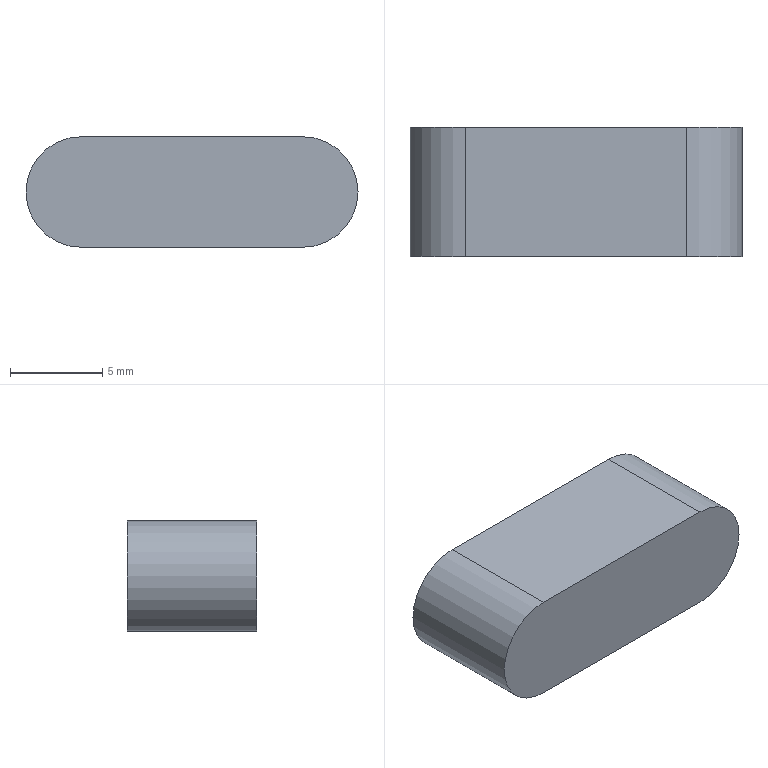Part | NX | features BREP 1 | 1 solid | 6 faces | box 18 x 7 x 6 mm | volume 701.92 mm3 | plane 4 | cylinder 2 | commonest cylinder face diameters 6 x2
STEP:
#1=CARTESIAN_POINT('',(0.,0.,-3.));
#2=VERTEX_POINT('',#1);
#3=CARTESIAN_POINT('',(0.,0.,3.));
#4=VERTEX_POINT('',#3);
#5=CARTESIAN_POINT('',(0.,0.,0.));
#6=DIRECTION('',(0.,1.,0.));
#7=DIRECTION('',(0.,0.,1.));
#8=AXIS2_PLACEMENT_3D('',#5,#6,#7);
#9=CIRCLE('',#8,3.);
#10=EDGE_CURVE('',#2,#4,#9,.T.);
#11=ORIENTED_EDGE('',*,*,#10,.T.);
#12=CARTESIAN_POINT('',(0.,7.,3.));
#13=VERTEX_POINT('',#12);
#14=CARTESIAN_POINT('',(0.,7.,3.));
#15=DIRECTION('',(0.,-1.,0.));
#16=VECTOR('',#15,1000.);
#17=LINE('',#14,#16);
#18=EDGE_CURVE('',#13,#4,#17,.T.);
#19=ORIENTED_EDGE('',*,*,#18,.F.);
#20=CARTESIAN_POINT('',(0.,7.,-3.));
#21=VERTEX_POINT('',#20);
#22=CARTESIAN_POINT('',(0.,7.,0.));
#23=DIRECTION('',(0.,1.,0.));
#24=DIRECTION('',(0.,0.,1.));
#25=AXIS2_PLACEMENT_3D('',#22,#23,#24);
#26=CIRCLE('',#25,3.);
#27=EDGE_CURVE('',#21,#13,#26,.T.);
#28=ORIENTED_EDGE('',*,*,#27,.F.);
#29=CARTESIAN_POINT('',(0.,7.,-3.));
#30=DIRECTION('',(0.,-1.,0.));
#31=VECTOR('',#30,1000.);
#32=LINE('',#29,#31);
#33=EDGE_CURVE('',#21,#2,#32,.T.);
#34=ORIENTED_EDGE('',*,*,#33,.T.);
#35=EDGE_LOOP('',(#11,#19,#28,#34));
#36=FACE_BOUND('',#35,.T.);
#37=CARTESIAN_POINT('',(0.,7.,0.));
#38=DIRECTION('',(0.,-1.,0.));
#39=DIRECTION('',(0.,0.,1.));
#40=AXIS2_PLACEMENT_3D('',#37,#38,#39);
#41=CYLINDRICAL_SURFACE('',#40,3.);
#42=ADVANCED_FACE('',(#36),#41,.T.);
#43=CARTESIAN_POINT('',(12.,0.,3.));
#44=VERTEX_POINT('',#43);
#45=CARTESIAN_POINT('',(0.,0.,3.));
#46=DIRECTION('',(1.,0.,0.));
#47=VECTOR('',#46,1000.);
#48=LINE('',#45,#47);
#49=EDGE_CURVE('',#4,#44,#48,.T.);
#50=ORIENTED_EDGE('',*,*,#49,.T.);
#51=CARTESIAN_POINT('',(12.,7.,3.));
#52=VERTEX_POINT('',#51);
#53=CARTESIAN_POINT('',(12.,7.,3.));
#54=DIRECTION('',(0.,-1.,0.));
#55=VECTOR('',#54,1000.);
#56=LINE('',#53,#55);
#57=EDGE_CURVE('',#52,#44,#56,.T.);
#58=ORIENTED_EDGE('',*,*,#57,.F.);
#59=CARTESIAN_POINT('',(0.,7.,3.));
#60=DIRECTION('',(1.,0.,0.));
#61=VECTOR('',#60,1000.);
#62=LINE('',#59,#61);
#63=EDGE_CURVE('',#13,#52,#62,.T.);
#64=ORIENTED_EDGE('',*,*,#63,.F.);
#65=ORIENTED_EDGE('',*,*,#18,.T.);
#66=EDGE_LOOP('',(#50,#58,#64,#65));
#67=FACE_BOUND('',#66,.T.);
#68=CARTESIAN_POINT('',(0.,7.,3.));
#69=DIRECTION('',(0.,0.,-1.));
#70=DIRECTION('',(0.,1.,0.));
#71=AXIS2_PLACEMENT_3D('',#68,#69,#70);
#72=PLANE('',#71);
#73=ADVANCED_FACE('',(#67),#72,.F.);
#74=CARTESIAN_POINT('',(12.,0.,-3.));
#75=VERTEX_POINT('',#74);
#76=CARTESIAN_POINT('',(12.,0.,0.));
#77=DIRECTION('',(0.,1.,0.));
#78=DIRECTION('',(0.,0.,1.));
#79=AXIS2_PLACEMENT_3D('',#76,#77,#78);
#80=CIRCLE('',#79,3.);
#81=EDGE_CURVE('',#44,#75,#80,.T.);
#82=ORIENTED_EDGE('',*,*,#81,.T.);
#83=CARTESIAN_POINT('',(12.,7.,-3.));
#84=VERTEX_POINT('',#83);
#85=CARTESIAN_POINT('',(12.,7.,-3.));
#86=DIRECTION('',(0.,-1.,0.));
#87=VECTOR('',#86,1000.);
#88=LINE('',#85,#87);
#89=EDGE_CURVE('',#84,#75,#88,.T.);
#90=ORIENTED_EDGE('',*,*,#89,.F.);
#91=CARTESIAN_POINT('',(12.,7.,0.));
#92=DIRECTION('',(0.,1.,0.));
#93=DIRECTION('',(0.,0.,1.));
#94=AXIS2_PLACEMENT_3D('',#91,#92,#93);
#95=CIRCLE('',#94,3.);
#96=EDGE_CURVE('',#52,#84,#95,.T.);
#97=ORIENTED_EDGE('',*,*,#96,.F.);
#98=ORIENTED_EDGE('',*,*,#57,.T.);
#99=EDGE_LOOP('',(#82,#90,#97,#98));
#100=FACE_BOUND('',#99,.T.);
#101=CARTESIAN_POINT('',(12.,7.,0.));
#102=DIRECTION('',(0.,-1.,0.));
#103=DIRECTION('',(0.,0.,1.));
#104=AXIS2_PLACEMENT_3D('',#101,#102,#103);
#105=CYLINDRICAL_SURFACE('',#104,3.);
#106=ADVANCED_FACE('',(#100),#105,.T.);
#107=CARTESIAN_POINT('',(0.,0.,-3.));
#108=DIRECTION('',(-1.,0.,0.));
#109=VECTOR('',#108,1000.);
#110=LINE('',#107,#109);
#111=EDGE_CURVE('',#75,#2,#110,.T.);
#112=ORIENTED_EDGE('',*,*,#111,.T.);
#113=ORIENTED_EDGE('',*,*,#33,.F.);
#114=CARTESIAN_POINT('',(0.,7.,-3.));
#115=DIRECTION('',(-1.,0.,0.));
#116=VECTOR('',#115,1000.);
#117=LINE('',#114,#116);
#118=EDGE_CURVE('',#84,#21,#117,.T.);
#119=ORIENTED_EDGE('',*,*,#118,.F.);
#120=ORIENTED_EDGE('',*,*,#89,.T.);
#121=EDGE_LOOP('',(#112,#113,#119,#120));
#122=FACE_BOUND('',#121,.T.);
#123=CARTESIAN_POINT('',(0.,7.,-3.));
#124=DIRECTION('',(0.,0.,1.));
#125=DIRECTION('',(-1.,0.,0.));
#126=AXIS2_PLACEMENT_3D('',#123,#124,#125);
#127=PLANE('',#126);
#128=ADVANCED_FACE('',(#122),#127,.F.);
#129=ORIENTED_EDGE('',*,*,#27,.T.);
#130=ORIENTED_EDGE('',*,*,#63,.T.);
#131=ORIENTED_EDGE('',*,*,#96,.T.);
#132=ORIENTED_EDGE('',*,*,#118,.T.);
#133=EDGE_LOOP('',(#129,#130,#131,#132));
#134=FACE_BOUND('',#133,.T.);
#135=CARTESIAN_POINT('',(0.,7.,0.));
#136=DIRECTION('',(0.,1.,0.));
#137=DIRECTION('',(-1.,0.,0.));
#138=AXIS2_PLACEMENT_3D('',#135,#136,#137);
#139=PLANE('',#138);
#140=ADVANCED_FACE('',(#134),#139,.T.);
#141=ORIENTED_EDGE('',*,*,#10,.F.);
#142=ORIENTED_EDGE('',*,*,#111,.F.);
#143=ORIENTED_EDGE('',*,*,#81,.F.);
#144=ORIENTED_EDGE('',*,*,#49,.F.);
#145=EDGE_LOOP('',(#141,#142,#143,#144));
#146=FACE_BOUND('',#145,.T.);
#147=CARTESIAN_POINT('',(0.,0.,0.));
#148=DIRECTION('',(0.,1.,0.));
#149=DIRECTION('',(-1.,0.,0.));
#150=AXIS2_PLACEMENT_3D('',#147,#148,#149);
#151=PLANE('',#150);
#152=ADVANCED_FACE('',(#146),#151,.F.);
#153=CLOSED_SHELL('',(#42,#73,#106,#128,#140,#152));
#154=MANIFOLD_SOLID_BREP('',#153);
#155=(LENGTH_UNIT()NAMED_UNIT(*)SI_UNIT(.MILLI.,.METRE.));
#156=UNCERTAINTY_MEASURE_WITH_UNIT(LENGTH_MEASURE(0.00001),#155,'','');
#157=(NAMED_UNIT(*)PLANE_ANGLE_UNIT()SI_UNIT($,.RADIAN.));
#158=(NAMED_UNIT(*)SI_UNIT($,.STERADIAN.)SOLID_ANGLE_UNIT());
#159=(GEOMETRIC_REPRESENTATION_CONTEXT(3)GLOBAL_UNCERTAINTY_ASSIGNED_CONTEXT((#156))GLOBAL_UNIT_ASSIGNED_CONTEXT((#155,#157,#158))REPRESENTATION_CONTEXT('',''));
#160=ADVANCED_BREP_SHAPE_REPRESENTATION('',(#154),#159);